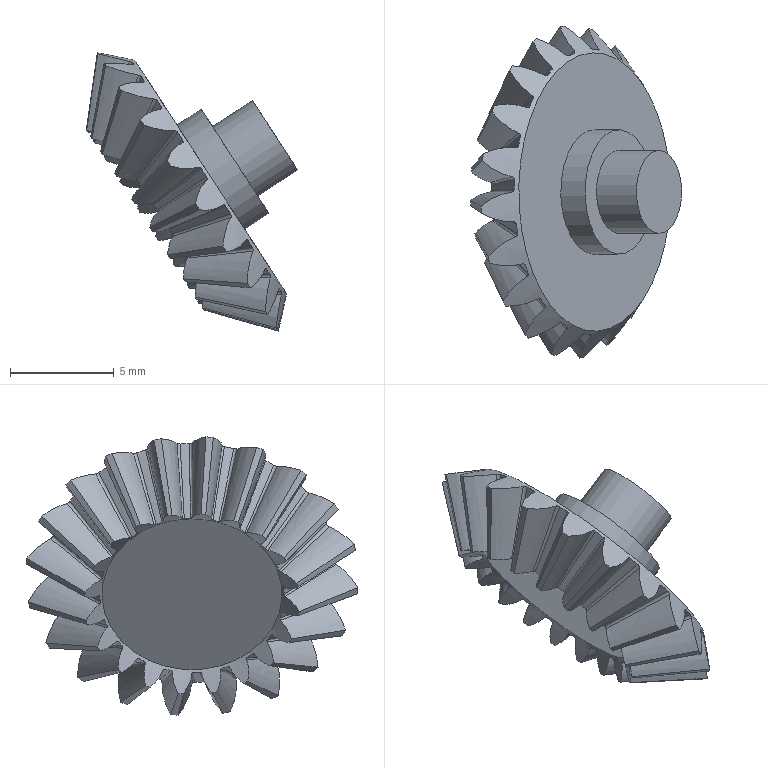Part | STEP file | Dodanie-wyci_gni_cie2_1 | 1 solid | 128 faces | box 10.182 x 16.004 x 13.419 mm | volume 470.763 mm3 | spline 108 | cone 14 | plane 4 | cylinder 2 | commonest cylinder face diameters 4 x1 6 x1